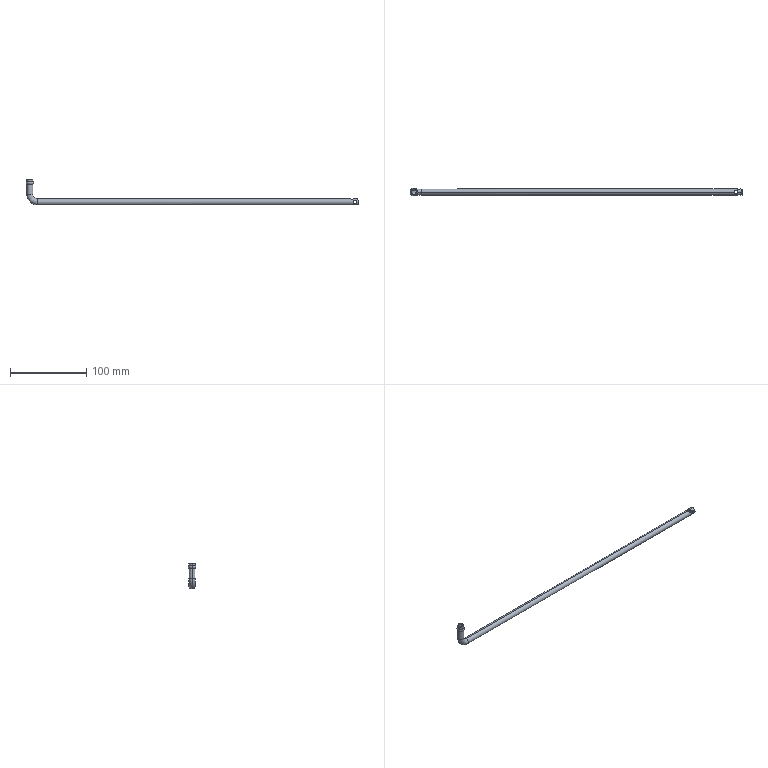Part | SolidWorks | features ICE 2, Fillet 1, Revolution 1, Sweep 1 | 1 solid | 30 faces | box 435 x 10 x 34 mm | volume 10005 mm3 | cylinder 18 | torus 10 | plane 2 | commonest cylinder face diameters 5 x8 8 x6 6 x4